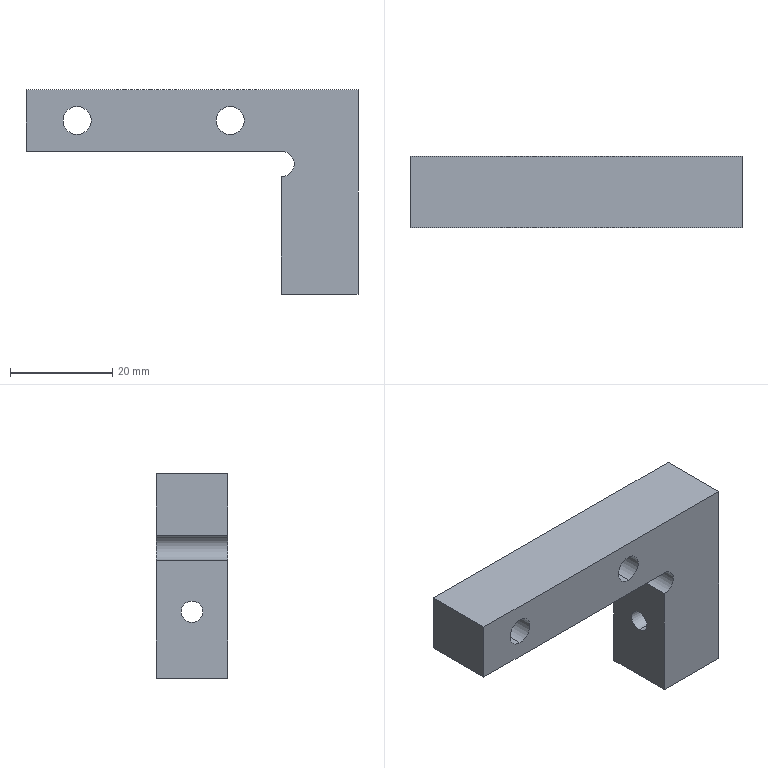Part | SolidWorks | features HoleWzd 2, ICE 2, Extrusion 1 | 1 solid | 21 faces | box 65 x 14 x 40 mm | volume 15165 mm3 | cylinder 11 | plane 10 | commonest cylinder face diameters 5.5 x4 10 x4 4.2 x2 5 x1
STEP:
#1=CARTESIAN_POINT('',(25.,0.,-23.1));
#2=VERTEX_POINT('',#1);
#3=CARTESIAN_POINT('',(25.,0.,-18.9));
#4=VERTEX_POINT('',#3);
#5=CARTESIAN_POINT('',(25.,0.,-21.));
#6=DIRECTION('',(-1.,0.,0.));
#7=DIRECTION('',(0.,0.,1.));
#8=AXIS2_PLACEMENT_3D('',#5,#6,#7);
#9=CIRCLE('',#8,2.1);
#10=EDGE_CURVE('',#2,#4,#9,.T.);
#11=ORIENTED_EDGE('',*,*,#10,.T.);
#12=CARTESIAN_POINT('',(40.,0.,-18.9));
#13=VERTEX_POINT('',#12);
#14=CARTESIAN_POINT('',(40.,0.,-18.9));
#15=DIRECTION('',(1.,0.,0.));
#16=VECTOR('',#15,1000.);
#17=LINE('',#14,#16);
#18=EDGE_CURVE('',#4,#13,#17,.T.);
#19=ORIENTED_EDGE('',*,*,#18,.T.);
#20=CARTESIAN_POINT('',(40.,0.,-23.1));
#21=VERTEX_POINT('',#20);
#22=CARTESIAN_POINT('',(40.,0.,-21.));
#23=DIRECTION('',(1.,0.,0.));
#24=DIRECTION('',(0.,0.,-1.));
#25=AXIS2_PLACEMENT_3D('',#22,#23,#24);
#26=CIRCLE('',#25,2.1);
#27=EDGE_CURVE('',#13,#21,#26,.T.);
#28=ORIENTED_EDGE('',*,*,#27,.T.);
#29=CARTESIAN_POINT('',(40.,0.,-23.1));
#30=DIRECTION('',(1.,0.,0.));
#31=VECTOR('',#30,1000.);
#32=LINE('',#29,#31);
#33=EDGE_CURVE('',#2,#21,#32,.T.);
#34=ORIENTED_EDGE('',*,*,#33,.F.);
#35=EDGE_LOOP('',(#11,#19,#28,#34));
#36=FACE_OUTER_BOUND('',#35,.T.);
#37=CARTESIAN_POINT('',(40.,0.,-21.));
#38=DIRECTION('',(1.,0.,0.));
#39=DIRECTION('',(0.,0.,-1.));
#40=AXIS2_PLACEMENT_3D('',#37,#38,#39);
#41=CYLINDRICAL_SURFACE('',#40,2.1);
#42=ADVANCED_FACE('',(#36),#41,.F.);
#43=CARTESIAN_POINT('',(-15.,1.3,-5.));
#44=VERTEX_POINT('',#43);
#45=CARTESIAN_POINT('',(-15.,1.3,5.));
#46=VERTEX_POINT('',#45);
#47=CARTESIAN_POINT('',(-15.,1.3,0.));
#48=DIRECTION('',(0.,1.,0.));
#49=DIRECTION('',(0.,0.,1.));
#50=AXIS2_PLACEMENT_3D('',#47,#48,#49);
#51=CIRCLE('',#50,5.);
#52=EDGE_CURVE('',#44,#46,#51,.T.);
#53=ORIENTED_EDGE('',*,*,#52,.F.);
#54=CARTESIAN_POINT('',(-15.,7.,-5.));
#55=VERTEX_POINT('',#54);
#56=CARTESIAN_POINT('',(-15.,7.,-5.));
#57=DIRECTION('',(0.,1.,0.));
#58=VECTOR('',#57,1000.);
#59=LINE('',#56,#58);
#60=EDGE_CURVE('',#44,#55,#59,.T.);
#61=ORIENTED_EDGE('',*,*,#60,.T.);
#62=CARTESIAN_POINT('',(-15.,7.,5.));
#63=VERTEX_POINT('',#62);
#64=CARTESIAN_POINT('',(-15.,7.,0.));
#65=DIRECTION('',(0.,1.,0.));
#66=DIRECTION('',(0.,0.,1.));
#67=AXIS2_PLACEMENT_3D('',#64,#65,#66);
#68=CIRCLE('',#67,5.);
#69=EDGE_CURVE('',#55,#63,#68,.T.);
#70=ORIENTED_EDGE('',*,*,#69,.T.);
#71=CARTESIAN_POINT('',(-15.,7.,5.));
#72=DIRECTION('',(0.,1.,0.));
#73=VECTOR('',#72,1000.);
#74=LINE('',#71,#73);
#75=EDGE_CURVE('',#46,#63,#74,.T.);
#76=ORIENTED_EDGE('',*,*,#75,.F.);
#77=EDGE_LOOP('',(#53,#61,#70,#76));
#78=FACE_OUTER_BOUND('',#77,.T.);
#79=CARTESIAN_POINT('',(-15.,7.,0.));
#80=DIRECTION('',(0.,1.,0.));
#81=DIRECTION('',(0.,0.,1.));
#82=AXIS2_PLACEMENT_3D('',#79,#80,#81);
#83=CYLINDRICAL_SURFACE('',#82,5.);
#84=ADVANCED_FACE('',(#78),#83,.F.);
#85=CARTESIAN_POINT('',(-15.,-7.,-2.75));
#86=VERTEX_POINT('',#85);
#87=CARTESIAN_POINT('',(-15.,-7.,2.75));
#88=VERTEX_POINT('',#87);
#89=CARTESIAN_POINT('',(-15.,-7.,0.));
#90=DIRECTION('',(0.,1.,0.));
#91=DIRECTION('',(0.,0.,1.));
#92=AXIS2_PLACEMENT_3D('',#89,#90,#91);
#93=CIRCLE('',#92,2.75);
#94=EDGE_CURVE('',#86,#88,#93,.T.);
#95=ORIENTED_EDGE('',*,*,#94,.F.);
#96=CARTESIAN_POINT('',(-15.,1.3,-2.75));
#97=VERTEX_POINT('',#96);
#98=CARTESIAN_POINT('',(-15.,7.,-2.75));
#99=DIRECTION('',(0.,1.,0.));
#100=VECTOR('',#99,1000.);
#101=LINE('',#98,#100);
#102=EDGE_CURVE('',#86,#97,#101,.T.);
#103=ORIENTED_EDGE('',*,*,#102,.T.);
#104=CARTESIAN_POINT('',(-15.,1.3,2.75));
#105=VERTEX_POINT('',#104);
#106=CARTESIAN_POINT('',(-15.,1.3,0.));
#107=DIRECTION('',(0.,1.,0.));
#108=DIRECTION('',(0.,0.,1.));
#109=AXIS2_PLACEMENT_3D('',#106,#107,#108);
#110=CIRCLE('',#109,2.75);
#111=EDGE_CURVE('',#97,#105,#110,.T.);
#112=ORIENTED_EDGE('',*,*,#111,.T.);
#113=CARTESIAN_POINT('',(-15.,7.,2.75));
#114=DIRECTION('',(0.,1.,0.));
#115=VECTOR('',#114,1000.);
#116=LINE('',#113,#115);
#117=EDGE_CURVE('',#88,#105,#116,.T.);
#118=ORIENTED_EDGE('',*,*,#117,.F.);
#119=EDGE_LOOP('',(#95,#103,#112,#118));
#120=FACE_OUTER_BOUND('',#119,.T.);
#121=CARTESIAN_POINT('',(-15.,7.,0.));
#122=DIRECTION('',(0.,1.,0.));
#123=DIRECTION('',(0.,0.,1.));
#124=AXIS2_PLACEMENT_3D('',#121,#122,#123);
#125=CYLINDRICAL_SURFACE('',#124,2.75);
#126=ADVANCED_FACE('',(#120),#125,.F.);
#127=CARTESIAN_POINT('',(15.,1.3,-5.));
#128=VERTEX_POINT('',#127);
#129=CARTESIAN_POINT('',(15.,1.3,5.));
#130=VERTEX_POINT('',#129);
#131=CARTESIAN_POINT('',(15.,1.3,0.));
#132=DIRECTION('',(0.,1.,0.));
#133=DIRECTION('',(0.,0.,1.));
#134=AXIS2_PLACEMENT_3D('',#131,#132,#133);
#135=CIRCLE('',#134,5.);
#136=EDGE_CURVE('',#128,#130,#135,.T.);
#137=ORIENTED_EDGE('',*,*,#136,.F.);
#138=CARTESIAN_POINT('',(15.,7.,-5.));
#139=VERTEX_POINT('',#138);
#140=CARTESIAN_POINT('',(15.,7.,-5.));
#141=DIRECTION('',(0.,1.,0.));
#142=VECTOR('',#141,1000.);
#143=LINE('',#140,#142);
#144=EDGE_CURVE('',#128,#139,#143,.T.);
#145=ORIENTED_EDGE('',*,*,#144,.T.);
#146=CARTESIAN_POINT('',(15.,7.,5.));
#147=VERTEX_POINT('',#146);
#148=CARTESIAN_POINT('',(15.,7.,0.));
#149=DIRECTION('',(0.,1.,0.));
#150=DIRECTION('',(0.,0.,1.));
#151=AXIS2_PLACEMENT_3D('',#148,#149,#150);
#152=CIRCLE('',#151,5.);
#153=EDGE_CURVE('',#139,#147,#152,.T.);
#154=ORIENTED_EDGE('',*,*,#153,.T.);
#155=CARTESIAN_POINT('',(15.,7.,5.));
#156=DIRECTION('',(0.,1.,0.));
#157=VECTOR('',#156,1000.);
#158=LINE('',#155,#157);
#159=EDGE_CURVE('',#130,#147,#158,.T.);
#160=ORIENTED_EDGE('',*,*,#159,.F.);
#161=EDGE_LOOP('',(#137,#145,#154,#160));
#162=FACE_OUTER_BOUND('',#161,.T.);
#163=CARTESIAN_POINT('',(15.,7.,0.));
#164=DIRECTION('',(0.,1.,0.));
#165=DIRECTION('',(0.,0.,1.));
#166=AXIS2_PLACEMENT_3D('',#163,#164,#165);
#167=CYLINDRICAL_SURFACE('',#166,5.);
#168=ADVANCED_FACE('',(#162),#167,.F.);
#169=CARTESIAN_POINT('',(15.,-7.,-2.75));
#170=VERTEX_POINT('',#169);
#171=CARTESIAN_POINT('',(15.,-7.,2.75));
#172=VERTEX_POINT('',#171);
#173=CARTESIAN_POINT('',(15.,-7.,0.));
#174=DIRECTION('',(0.,1.,0.));
#175=DIRECTION('',(0.,0.,1.));
#176=AXIS2_PLACEMENT_3D('',#173,#174,#175);
#177=CIRCLE('',#176,2.75);
#178=EDGE_CURVE('',#170,#172,#177,.T.);
#179=ORIENTED_EDGE('',*,*,#178,.F.);
#180=CARTESIAN_POINT('',(15.,1.3,-2.75));
#181=VERTEX_POINT('',#180);
#182=CARTESIAN_POINT('',(15.,7.,-2.75));
#183=DIRECTION('',(0.,1.,0.));
#184=VECTOR('',#183,1000.);
#185=LINE('',#182,#184);
#186=EDGE_CURVE('',#170,#181,#185,.T.);
#187=ORIENTED_EDGE('',*,*,#186,.T.);
#188=CARTESIAN_POINT('',(15.,1.3,2.75));
#189=VERTEX_POINT('',#188);
#190=CARTESIAN_POINT('',(15.,1.3,0.));
#191=DIRECTION('',(0.,1.,0.));
#192=DIRECTION('',(0.,0.,1.));
#193=AXIS2_PLACEMENT_3D('',#190,#191,#192);
#194=CIRCLE('',#193,2.75);
#195=EDGE_CURVE('',#181,#189,#194,.T.);
#196=ORIENTED_EDGE('',*,*,#195,.T.);
#197=CARTESIAN_POINT('',(15.,7.,2.75));
#198=DIRECTION('',(0.,1.,0.));
#199=VECTOR('',#198,1000.);
#200=LINE('',#197,#199);
#201=EDGE_CURVE('',#172,#189,#200,.T.);
#202=ORIENTED_EDGE('',*,*,#201,.F.);
#203=EDGE_LOOP('',(#179,#187,#196,#202));
#204=FACE_OUTER_BOUND('',#203,.T.);
#205=CARTESIAN_POINT('',(15.,7.,0.));
#206=DIRECTION('',(0.,1.,0.));
#207=DIRECTION('',(0.,0.,1.));
#208=AXIS2_PLACEMENT_3D('',#205,#206,#207);
#209=CYLINDRICAL_SURFACE('',#208,2.75);
#210=ADVANCED_FACE('',(#204),#209,.F.);
#211=CARTESIAN_POINT('',(25.,-7.,-6.));
#212=VERTEX_POINT('',#211);
#213=CARTESIAN_POINT('',(-25.,-7.,-6.));
#214=VERTEX_POINT('',#213);
#215=CARTESIAN_POINT('',(-25.,-7.,-6.));
#216=DIRECTION('',(-1.,0.,0.));
#217=VECTOR('',#216,1000.);
#218=LINE('',#215,#217);
#219=EDGE_CURVE('',#212,#214,#218,.T.);
#220=ORIENTED_EDGE('',*,*,#219,.T.);
#221=CARTESIAN_POINT('',(-25.,7.,-6.));
#222=VERTEX_POINT('',#221);
#223=CARTESIAN_POINT('',(-25.,7.,-6.));
#224=DIRECTION('',(0.,-1.,0.));
#225=VECTOR('',#224,1000.);
#226=LINE('',#223,#225);
#227=EDGE_CURVE('',#222,#214,#226,.T.);
#228=ORIENTED_EDGE('',*,*,#227,.F.);
#229=CARTESIAN_POINT('',(25.,7.,-6.));
#230=VERTEX_POINT('',#229);
#231=CARTESIAN_POINT('',(-25.,7.,-6.));
#232=DIRECTION('',(-1.,0.,0.));
#233=VECTOR('',#232,1000.);
#234=LINE('',#231,#233);
#235=EDGE_CURVE('',#230,#222,#234,.T.);
#236=ORIENTED_EDGE('',*,*,#235,.F.);
#237=CARTESIAN_POINT('',(25.,7.,-6.));
#238=DIRECTION('',(0.,-1.,0.));
#239=VECTOR('',#238,1000.);
#240=LINE('',#237,#239);
#241=EDGE_CURVE('',#230,#212,#240,.T.);
#242=ORIENTED_EDGE('',*,*,#241,.T.);
#243=EDGE_LOOP('',(#220,#228,#236,#242));
#244=FACE_OUTER_BOUND('',#243,.T.);
#245=CARTESIAN_POINT('',(-25.,7.,-6.));
#246=DIRECTION('',(0.,0.,1.));
#247=DIRECTION('',(1.,0.,0.));
#248=AXIS2_PLACEMENT_3D('',#245,#246,#247);
#249=PLANE('',#248);
#250=ADVANCED_FACE('',(#244),#249,.F.);
#251=CARTESIAN_POINT('',(-25.,-7.,6.));
#252=VERTEX_POINT('',#251);
#253=CARTESIAN_POINT('',(-25.,-7.,6.));
#254=DIRECTION('',(0.,0.,1.));
#255=VECTOR('',#254,1000.);
#256=LINE('',#253,#255);
#257=EDGE_CURVE('',#214,#252,#256,.T.);
#258=ORIENTED_EDGE('',*,*,#257,.T.);
#259=CARTESIAN_POINT('',(-25.,7.,6.));
#260=VERTEX_POINT('',#259);
#261=CARTESIAN_POINT('',(-25.,7.,6.));
#262=DIRECTION('',(0.,-1.,0.));
#263=VECTOR('',#262,1000.);
#264=LINE('',#261,#263);
#265=EDGE_CURVE('',#260,#252,#264,.T.);
#266=ORIENTED_EDGE('',*,*,#265,.F.);
#267=CARTESIAN_POINT('',(-25.,7.,6.));
#268=DIRECTION('',(0.,0.,1.));
#269=VECTOR('',#268,1000.);
#270=LINE('',#267,#269);
#271=EDGE_CURVE('',#222,#260,#270,.T.);
#272=ORIENTED_EDGE('',*,*,#271,.F.);
#273=ORIENTED_EDGE('',*,*,#227,.T.);
#274=EDGE_LOOP('',(#258,#266,#272,#273));
#275=FACE_OUTER_BOUND('',#274,.T.);
#276=CARTESIAN_POINT('',(-25.,7.,6.));
#277=DIRECTION('',(1.,0.,0.));
#278=DIRECTION('',(0.,0.,-1.));
#279=AXIS2_PLACEMENT_3D('',#276,#277,#278);
#280=PLANE('',#279);
#281=ADVANCED_FACE('',(#275),#280,.F.);
#282=CARTESIAN_POINT('',(40.,-7.,6.));
#283=VERTEX_POINT('',#282);
#284=CARTESIAN_POINT('',(-25.,-7.,6.));
#285=DIRECTION('',(1.,0.,0.));
#286=VECTOR('',#285,1000.);
#287=LINE('',#284,#286);
#288=EDGE_CURVE('',#252,#283,#287,.T.);
#289=ORIENTED_EDGE('',*,*,#288,.T.);
#290=CARTESIAN_POINT('',(40.,7.,6.));
#291=VERTEX_POINT('',#290);
#292=CARTESIAN_POINT('',(40.,-49.72,6.));
#293=DIRECTION('',(0.,1.,0.));
#294=VECTOR('',#293,1000.);
#295=LINE('',#292,#294);
#296=EDGE_CURVE('',#283,#291,#295,.T.);
#297=ORIENTED_EDGE('',*,*,#296,.T.);
#298=CARTESIAN_POINT('',(-25.,7.,6.));
#299=DIRECTION('',(1.,0.,0.));
#300=VECTOR('',#299,1000.);
#301=LINE('',#298,#300);
#302=EDGE_CURVE('',#260,#291,#301,.T.);
#303=ORIENTED_EDGE('',*,*,#302,.F.);
#304=ORIENTED_EDGE('',*,*,#265,.T.);
#305=EDGE_LOOP('',(#289,#297,#303,#304));
#306=FACE_OUTER_BOUND('',#305,.T.);
#307=CARTESIAN_POINT('',(-25.,7.,6.));
#308=DIRECTION('',(0.,0.,-1.));
#309=DIRECTION('',(-1.,0.,0.));
#310=AXIS2_PLACEMENT_3D('',#307,#308,#309);
#311=PLANE('',#310);
#312=ADVANCED_FACE('',(#306),#311,.F.);
#313=CARTESIAN_POINT('',(-15.,7.,0.));
#314=DIRECTION('',(0.,1.,0.));
#315=DIRECTION('',(0.,0.,1.));
#316=AXIS2_PLACEMENT_3D('',#313,#314,#315);
#317=CIRCLE('',#316,5.);
#318=EDGE_CURVE('',#63,#55,#317,.T.);
#319=ORIENTED_EDGE('',*,*,#318,.F.);
#320=ORIENTED_EDGE('',*,*,#69,.F.);
#321=EDGE_LOOP('',(#319,#320));
#322=FACE_BOUND('',#321,.T.);
#323=CARTESIAN_POINT('',(15.,7.,0.));
#324=DIRECTION('',(0.,1.,0.));
#325=DIRECTION('',(0.,0.,1.));
#326=AXIS2_PLACEMENT_3D('',#323,#324,#325);
#327=CIRCLE('',#326,5.);
#328=EDGE_CURVE('',#147,#139,#327,.T.);
#329=ORIENTED_EDGE('',*,*,#328,.F.);
#330=ORIENTED_EDGE('',*,*,#153,.F.);
#331=EDGE_LOOP('',(#329,#330));
#332=FACE_BOUND('',#331,.T.);
#333=CARTESIAN_POINT('',(25.,7.,-34.));
#334=VERTEX_POINT('',#333);
#335=CARTESIAN_POINT('',(25.,7.,-11.));
#336=VERTEX_POINT('',#335);
#337=CARTESIAN_POINT('',(25.,7.,6.));
#338=DIRECTION('',(0.,0.,1.));
#339=VECTOR('',#338,1000.);
#340=LINE('',#337,#339);
#341=EDGE_CURVE('',#334,#336,#340,.T.);
#342=ORIENTED_EDGE('',*,*,#341,.T.);
#343=CARTESIAN_POINT('',(25.,7.,-8.5));
#344=DIRECTION('',(0.,1.,0.));
#345=DIRECTION('',(0.,0.,1.));
#346=AXIS2_PLACEMENT_3D('',#343,#344,#345);
#347=CIRCLE('',#346,2.5);
#348=EDGE_CURVE('',#230,#336,#347,.T.);
#349=ORIENTED_EDGE('',*,*,#348,.F.);
#350=ORIENTED_EDGE('',*,*,#235,.T.);
#351=ORIENTED_EDGE('',*,*,#271,.T.);
#352=ORIENTED_EDGE('',*,*,#302,.T.);
#353=CARTESIAN_POINT('',(40.,7.,-34.));
#354=VERTEX_POINT('',#353);
#355=CARTESIAN_POINT('',(40.,7.,6.));
#356=DIRECTION('',(0.,0.,-1.));
#357=VECTOR('',#356,1000.);
#358=LINE('',#355,#357);
#359=EDGE_CURVE('',#291,#354,#358,.T.);
#360=ORIENTED_EDGE('',*,*,#359,.T.);
#361=CARTESIAN_POINT('',(25.,7.,-34.));
#362=DIRECTION('',(-1.,0.,0.));
#363=VECTOR('',#362,1000.);
#364=LINE('',#361,#363);
#365=EDGE_CURVE('',#354,#334,#364,.T.);
#366=ORIENTED_EDGE('',*,*,#365,.T.);
#367=EDGE_LOOP('',(#342,#349,#350,#351,#352,#360,#366));
#368=FACE_OUTER_BOUND('',#367,.T.);
#369=CARTESIAN_POINT('',(0.,7.,0.));
#370=DIRECTION('',(0.,-1.,0.));
#371=DIRECTION('',(0.,0.,-1.));
#372=AXIS2_PLACEMENT_3D('',#369,#370,#371);
#373=PLANE('',#372);
#374=ADVANCED_FACE('',(#322,#332,#368),#373,.F.);
#375=CARTESIAN_POINT('',(25.,-7.,-11.));
#376=VERTEX_POINT('',#375);
#377=CARTESIAN_POINT('',(25.,-7.,-8.5));
#378=DIRECTION('',(0.,1.,0.));
#379=DIRECTION('',(0.,0.,1.));
#380=AXIS2_PLACEMENT_3D('',#377,#378,#379);
#381=CIRCLE('',#380,2.5);
#382=EDGE_CURVE('',#212,#376,#381,.T.);
#383=ORIENTED_EDGE('',*,*,#382,.T.);
#384=CARTESIAN_POINT('',(25.,-7.,-34.));
#385=VERTEX_POINT('',#384);
#386=CARTESIAN_POINT('',(25.,-7.,6.));
#387=DIRECTION('',(0.,0.,1.));
#388=VECTOR('',#387,1000.);
#389=LINE('',#386,#388);
#390=EDGE_CURVE('',#385,#376,#389,.T.);
#391=ORIENTED_EDGE('',*,*,#390,.F.);
#392=CARTESIAN_POINT('',(40.,-7.,-34.));
#393=VERTEX_POINT('',#392);
#394=CARTESIAN_POINT('',(25.,-7.,-34.));
#395=DIRECTION('',(-1.,0.,0.));
#396=VECTOR('',#395,1000.);
#397=LINE('',#394,#396);
#398=EDGE_CURVE('',#393,#385,#397,.T.);
#399=ORIENTED_EDGE('',*,*,#398,.F.);
#400=CARTESIAN_POINT('',(40.,-7.,6.));
#401=DIRECTION('',(0.,0.,-1.));
#402=VECTOR('',#401,1000.);
#403=LINE('',#400,#402);
#404=EDGE_CURVE('',#283,#393,#403,.T.);
#405=ORIENTED_EDGE('',*,*,#404,.F.);
#406=ORIENTED_EDGE('',*,*,#288,.F.);
#407=ORIENTED_EDGE('',*,*,#257,.F.);
#408=ORIENTED_EDGE('',*,*,#219,.F.);
#409=EDGE_LOOP('',(#383,#391,#399,#405,#406,#407,#408));
#410=FACE_OUTER_BOUND('',#409,.T.);
#411=CARTESIAN_POINT('',(-15.,-7.,0.));
#412=DIRECTION('',(0.,1.,0.));
#413=DIRECTION('',(0.,0.,1.));
#414=AXIS2_PLACEMENT_3D('',#411,#412,#413);
#415=CIRCLE('',#414,2.75);
#416=EDGE_CURVE('',#88,#86,#415,.T.);
#417=ORIENTED_EDGE('',*,*,#416,.T.);
#418=ORIENTED_EDGE('',*,*,#94,.T.);
#419=EDGE_LOOP('',(#417,#418));
#420=FACE_BOUND('',#419,.T.);
#421=CARTESIAN_POINT('',(15.,-7.,0.));
#422=DIRECTION('',(0.,1.,0.));
#423=DIRECTION('',(0.,0.,1.));
#424=AXIS2_PLACEMENT_3D('',#421,#422,#423);
#425=CIRCLE('',#424,2.75);
#426=EDGE_CURVE('',#172,#170,#425,.T.);
#427=ORIENTED_EDGE('',*,*,#426,.T.);
#428=ORIENTED_EDGE('',*,*,#178,.T.);
#429=EDGE_LOOP('',(#427,#428));
#430=FACE_BOUND('',#429,.T.);
#431=CARTESIAN_POINT('',(0.,-7.,0.));
#432=DIRECTION('',(0.,-1.,0.));
#433=DIRECTION('',(0.,0.,-1.));
#434=AXIS2_PLACEMENT_3D('',#431,#432,#433);
#435=PLANE('',#434);
#436=ADVANCED_FACE('',(#410,#420,#430),#435,.T.);
#437=ORIENTED_EDGE('',*,*,#186,.F.);
#438=ORIENTED_EDGE('',*,*,#426,.F.);
#439=ORIENTED_EDGE('',*,*,#201,.T.);
#440=CARTESIAN_POINT('',(15.,1.3,0.));
#441=DIRECTION('',(0.,1.,0.));
#442=DIRECTION('',(0.,0.,1.));
#443=AXIS2_PLACEMENT_3D('',#440,#441,#442);
#444=CIRCLE('',#443,2.75);
#445=EDGE_CURVE('',#189,#181,#444,.T.);
#446=ORIENTED_EDGE('',*,*,#445,.T.);
#447=EDGE_LOOP('',(#437,#438,#439,#446));
#448=FACE_OUTER_BOUND('',#447,.T.);
#449=CARTESIAN_POINT('',(15.,7.,0.));
#450=DIRECTION('',(0.,1.,0.));
#451=DIRECTION('',(0.,0.,1.));
#452=AXIS2_PLACEMENT_3D('',#449,#450,#451);
#453=CYLINDRICAL_SURFACE('',#452,2.75);
#454=ADVANCED_FACE('',(#448),#453,.F.);
#455=ORIENTED_EDGE('',*,*,#445,.F.);
#456=ORIENTED_EDGE('',*,*,#195,.F.);
#457=EDGE_LOOP('',(#455,#456));
#458=FACE_BOUND('',#457,.T.);
#459=CARTESIAN_POINT('',(15.,1.3,0.));
#460=DIRECTION('',(0.,1.,0.));
#461=DIRECTION('',(0.,0.,1.));
#462=AXIS2_PLACEMENT_3D('',#459,#460,#461);
#463=CIRCLE('',#462,5.);
#464=EDGE_CURVE('',#130,#128,#463,.T.);
#465=ORIENTED_EDGE('',*,*,#464,.T.);
#466=ORIENTED_EDGE('',*,*,#136,.T.);
#467=EDGE_LOOP('',(#465,#466));
#468=FACE_OUTER_BOUND('',#467,.T.);
#469=CARTESIAN_POINT('',(17.75,1.3,0.));
#470=DIRECTION('',(0.,-1.,0.));
#471=DIRECTION('',(0.,0.,-1.));
#472=AXIS2_PLACEMENT_3D('',#469,#470,#471);
#473=PLANE('',#472);
#474=ADVANCED_FACE('',(#458,#468),#473,.F.);
#475=ORIENTED_EDGE('',*,*,#144,.F.);
#476=ORIENTED_EDGE('',*,*,#464,.F.);
#477=ORIENTED_EDGE('',*,*,#159,.T.);
#478=ORIENTED_EDGE('',*,*,#328,.T.);
#479=EDGE_LOOP('',(#475,#476,#477,#478));
#480=FACE_OUTER_BOUND('',#479,.T.);
#481=CARTESIAN_POINT('',(15.,7.,0.));
#482=DIRECTION('',(0.,1.,0.));
#483=DIRECTION('',(0.,0.,1.));
#484=AXIS2_PLACEMENT_3D('',#481,#482,#483);
#485=CYLINDRICAL_SURFACE('',#484,5.);
#486=ADVANCED_FACE('',(#480),#485,.F.);
#487=ORIENTED_EDGE('',*,*,#102,.F.);
#488=ORIENTED_EDGE('',*,*,#416,.F.);
#489=ORIENTED_EDGE('',*,*,#117,.T.);
#490=CARTESIAN_POINT('',(-15.,1.3,0.));
#491=DIRECTION('',(0.,1.,0.));
#492=DIRECTION('',(0.,0.,1.));
#493=AXIS2_PLACEMENT_3D('',#490,#491,#492);
#494=CIRCLE('',#493,2.75);
#495=EDGE_CURVE('',#105,#97,#494,.T.);
#496=ORIENTED_EDGE('',*,*,#495,.T.);
#497=EDGE_LOOP('',(#487,#488,#489,#496));
#498=FACE_OUTER_BOUND('',#497,.T.);
#499=CARTESIAN_POINT('',(-15.,7.,0.));
#500=DIRECTION('',(0.,1.,0.));
#501=DIRECTION('',(0.,0.,1.));
#502=AXIS2_PLACEMENT_3D('',#499,#500,#501);
#503=CYLINDRICAL_SURFACE('',#502,2.75);
#504=ADVANCED_FACE('',(#498),#503,.F.);
#505=ORIENTED_EDGE('',*,*,#495,.F.);
#506=ORIENTED_EDGE('',*,*,#111,.F.);
#507=EDGE_LOOP('',(#505,#506));
#508=FACE_BOUND('',#507,.T.);
#509=CARTESIAN_POINT('',(-15.,1.3,0.));
#510=DIRECTION('',(0.,1.,0.));
#511=DIRECTION('',(0.,0.,1.));
#512=AXIS2_PLACEMENT_3D('',#509,#510,#511);
#513=CIRCLE('',#512,5.);
#514=EDGE_CURVE('',#46,#44,#513,.T.);
#515=ORIENTED_EDGE('',*,*,#514,.T.);
#516=ORIENTED_EDGE('',*,*,#52,.T.);
#517=EDGE_LOOP('',(#515,#516));
#518=FACE_OUTER_BOUND('',#517,.T.);
#519=CARTESIAN_POINT('',(-12.25,1.3,0.));
#520=DIRECTION('',(0.,-1.,0.));
#521=DIRECTION('',(0.,0.,-1.));
#522=AXIS2_PLACEMENT_3D('',#519,#520,#521);
#523=PLANE('',#522);
#524=ADVANCED_FACE('',(#508,#518),#523,.F.);
#525=ORIENTED_EDGE('',*,*,#60,.F.);
#526=ORIENTED_EDGE('',*,*,#514,.F.);
#527=ORIENTED_EDGE('',*,*,#75,.T.);
#528=ORIENTED_EDGE('',*,*,#318,.T.);
#529=EDGE_LOOP('',(#525,#526,#527,#528));
#530=FACE_OUTER_BOUND('',#529,.T.);
#531=CARTESIAN_POINT('',(-15.,7.,0.));
#532=DIRECTION('',(0.,1.,0.));
#533=DIRECTION('',(0.,0.,1.));
#534=AXIS2_PLACEMENT_3D('',#531,#532,#533);
#535=CYLINDRICAL_SURFACE('',#534,5.);
#536=ADVANCED_FACE('',(#530),#535,.F.);
#537=CARTESIAN_POINT('',(25.,-7.,-11.));
#538=DIRECTION('',(0.,-1.,0.));
#539=VECTOR('',#538,1000.);
#540=LINE('',#537,#539);
#541=EDGE_CURVE('',#336,#376,#540,.T.);
#542=ORIENTED_EDGE('',*,*,#541,.F.);
#543=ORIENTED_EDGE('',*,*,#341,.F.);
#544=CARTESIAN_POINT('',(25.,-49.72,-34.));
#545=DIRECTION('',(0.,1.,0.));
#546=VECTOR('',#545,1000.);
#547=LINE('',#544,#546);
#548=EDGE_CURVE('',#385,#334,#547,.T.);
#549=ORIENTED_EDGE('',*,*,#548,.F.);
#550=ORIENTED_EDGE('',*,*,#390,.T.);
#551=EDGE_LOOP('',(#542,#543,#549,#550));
#552=FACE_OUTER_BOUND('',#551,.T.);
#553=ORIENTED_EDGE('',*,*,#10,.F.);
#554=CARTESIAN_POINT('',(25.,0.,-21.));
#555=DIRECTION('',(-1.,0.,0.));
#556=DIRECTION('',(0.,0.,1.));
#557=AXIS2_PLACEMENT_3D('',#554,#555,#556);
#558=CIRCLE('',#557,2.1);
#559=EDGE_CURVE('',#4,#2,#558,.T.);
#560=ORIENTED_EDGE('',*,*,#559,.F.);
#561=EDGE_LOOP('',(#553,#560));
#562=FACE_BOUND('',#561,.T.);
#563=CARTESIAN_POINT('',(25.,-49.72,6.));
#564=DIRECTION('',(-1.,0.,0.));
#565=DIRECTION('',(0.,0.,1.));
#566=AXIS2_PLACEMENT_3D('',#563,#564,#565);
#567=PLANE('',#566);
#568=ADVANCED_FACE('',(#552,#562),#567,.T.);
#569=CARTESIAN_POINT('',(40.,0.,-21.));
#570=DIRECTION('',(1.,0.,0.));
#571=DIRECTION('',(0.,0.,-1.));
#572=AXIS2_PLACEMENT_3D('',#569,#570,#571);
#573=CIRCLE('',#572,2.1);
#574=EDGE_CURVE('',#21,#13,#573,.T.);
#575=ORIENTED_EDGE('',*,*,#574,.F.);
#576=ORIENTED_EDGE('',*,*,#27,.F.);
#577=EDGE_LOOP('',(#575,#576));
#578=FACE_BOUND('',#577,.T.);
#579=ORIENTED_EDGE('',*,*,#296,.F.);
#580=ORIENTED_EDGE('',*,*,#404,.T.);
#581=CARTESIAN_POINT('',(40.,-49.72,-34.));
#582=DIRECTION('',(0.,1.,0.));
#583=VECTOR('',#582,1000.);
#584=LINE('',#581,#583);
#585=EDGE_CURVE('',#393,#354,#584,.T.);
#586=ORIENTED_EDGE('',*,*,#585,.T.);
#587=ORIENTED_EDGE('',*,*,#359,.F.);
#588=EDGE_LOOP('',(#579,#580,#586,#587));
#589=FACE_OUTER_BOUND('',#588,.T.);
#590=CARTESIAN_POINT('',(40.,-49.72,6.));
#591=DIRECTION('',(1.,0.,0.));
#592=DIRECTION('',(0.,0.,-1.));
#593=AXIS2_PLACEMENT_3D('',#590,#591,#592);
#594=PLANE('',#593);
#595=ADVANCED_FACE('',(#578,#589),#594,.T.);
#596=ORIENTED_EDGE('',*,*,#585,.F.);
#597=ORIENTED_EDGE('',*,*,#398,.T.);
#598=ORIENTED_EDGE('',*,*,#548,.T.);
#599=ORIENTED_EDGE('',*,*,#365,.F.);
#600=EDGE_LOOP('',(#596,#597,#598,#599));
#601=FACE_OUTER_BOUND('',#600,.T.);
#602=CARTESIAN_POINT('',(25.,-49.72,-34.));
#603=DIRECTION('',(0.,0.,-1.));
#604=DIRECTION('',(-1.,0.,0.));
#605=AXIS2_PLACEMENT_3D('',#602,#603,#604);
#606=PLANE('',#605);
#607=ADVANCED_FACE('',(#601),#606,.T.);
#608=ORIENTED_EDGE('',*,*,#18,.F.);
#609=ORIENTED_EDGE('',*,*,#559,.T.);
#610=ORIENTED_EDGE('',*,*,#33,.T.);
#611=ORIENTED_EDGE('',*,*,#574,.T.);
#612=EDGE_LOOP('',(#608,#609,#610,#611));
#613=FACE_OUTER_BOUND('',#612,.T.);
#614=CARTESIAN_POINT('',(40.,0.,-21.));
#615=DIRECTION('',(1.,0.,0.));
#616=DIRECTION('',(0.,0.,-1.));
#617=AXIS2_PLACEMENT_3D('',#614,#615,#616);
#618=CYLINDRICAL_SURFACE('',#617,2.1);
#619=ADVANCED_FACE('',(#613),#618,.F.);
#620=ORIENTED_EDGE('',*,*,#241,.F.);
#621=ORIENTED_EDGE('',*,*,#348,.T.);
#622=ORIENTED_EDGE('',*,*,#541,.T.);
#623=ORIENTED_EDGE('',*,*,#382,.F.);
#624=EDGE_LOOP('',(#620,#621,#622,#623));
#625=FACE_OUTER_BOUND('',#624,.T.);
#626=CARTESIAN_POINT('',(25.,-7.,-8.5));
#627=DIRECTION('',(0.,1.,0.));
#628=DIRECTION('',(0.,0.,1.));
#629=AXIS2_PLACEMENT_3D('',#626,#627,#628);
#630=CYLINDRICAL_SURFACE('',#629,2.5);
#631=ADVANCED_FACE('',(#625),#630,.F.);
#632=CLOSED_SHELL('',(#42,#84,#126,#168,#210,#250,#281,#312,#374,#436,#454,#474,#486,#504,#524,#536,#568,#595,#607,#619,#631));
#633=MANIFOLD_SOLID_BREP('',#632);
#634=CARTESIAN_POINT('',(0.,0.,0.));
#635=DIRECTION('',(0.,0.,1.));
#636=DIRECTION('',(1.,0.,0.));
#637=AXIS2_PLACEMENT_3D('',#634,#635,#636);
#638=(LENGTH_UNIT()NAMED_UNIT(*)SI_UNIT(.MILLI.,.METRE.));
#639=UNCERTAINTY_MEASURE_WITH_UNIT(LENGTH_MEASURE(0.00001),#638,'','');
#640=(NAMED_UNIT(*)PLANE_ANGLE_UNIT()SI_UNIT($,.RADIAN.));
#641=(NAMED_UNIT(*)SI_UNIT($,.STERADIAN.)SOLID_ANGLE_UNIT());
#642=(GEOMETRIC_REPRESENTATION_CONTEXT(3)GLOBAL_UNCERTAINTY_ASSIGNED_CONTEXT((#639))GLOBAL_UNIT_ASSIGNED_CONTEXT((#638,#640,#641))REPRESENTATION_CONTEXT('',''));
#643=ADVANCED_BREP_SHAPE_REPRESENTATION('',(#633,#637),#642);